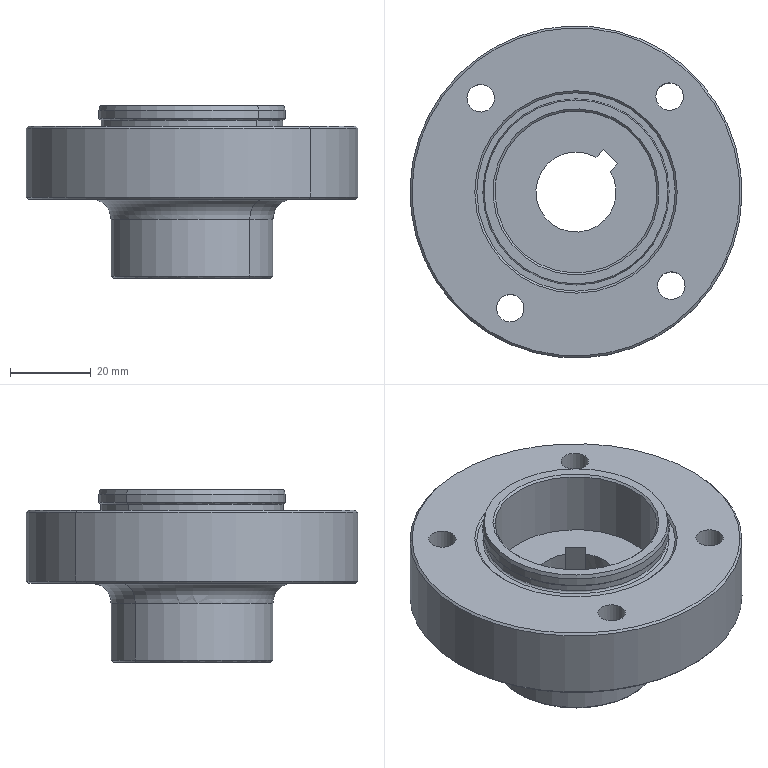Part | SolidWorks | features BaseBody 1 | 1 solid | 48 faces | box 82 x 82 x 42.5 mm | volume 94229 mm3 | cylinder 18 | cone 17 | plane 9 | torus 4 | commonest cylinder face diameters 6.8 x8 40 x4 45 x2 46 x2 82 x2
STEP:
#1=CARTESIAN_POINT('',(-51.524,-43.165,125.25));
#2=VERTEX_POINT('',#1);
#3=CARTESIAN_POINT('',(-37.402,-57.043,125.25));
#4=VERTEX_POINT('',#3);
#5=CARTESIAN_POINT('',(-44.463,-50.104,125.25));
#6=DIRECTION('',(0.,0.,1.));
#7=DIRECTION('',(0.7133,-0.7009,0.));
#8=AXIS2_PLACEMENT_3D('',#5,#6,#7);
#9=CIRCLE('',#8,9.9);
#10=EDGE_CURVE('',#2,#4,#9,.T.);
#11=ORIENTED_EDGE('',*,*,#10,.T.);
#12=CARTESIAN_POINT('',(-35.547,-58.865,99.25));
#13=VERTEX_POINT('',#12);
#14=CARTESIAN_POINT('',(-37.402,-57.043,125.25));
#15=DIRECTION('',(0.07097,-0.06974,-0.995));
#16=VECTOR('',#15,1000.);
#17=LINE('',#14,#16);
#18=EDGE_CURVE('',#4,#13,#17,.T.);
#19=ORIENTED_EDGE('',*,*,#18,.T.);
#20=CARTESIAN_POINT('',(-53.379,-41.342,99.25));
#21=VERTEX_POINT('',#20);
#22=CARTESIAN_POINT('',(-44.463,-50.104,99.25));
#23=DIRECTION('',(0.,0.,1.));
#24=DIRECTION('',(0.7133,-0.7009,0.));
#25=AXIS2_PLACEMENT_3D('',#22,#23,#24);
#26=CIRCLE('',#25,12.5);
#27=EDGE_CURVE('',#21,#13,#26,.T.);
#28=ORIENTED_EDGE('',*,*,#27,.F.);
#29=CARTESIAN_POINT('',(-51.524,-43.165,125.25));
#30=DIRECTION('',(-0.07097,0.06974,-0.995));
#31=VECTOR('',#30,1000.);
#32=LINE('',#29,#31);
#33=EDGE_CURVE('',#2,#21,#32,.T.);
#34=ORIENTED_EDGE('',*,*,#33,.F.);
#35=EDGE_LOOP('',(#11,#19,#28,#34));
#36=FACE_OUTER_BOUND('',#35,.T.);
#37=CARTESIAN_POINT('',(-44.463,-50.104,125.25));
#38=DIRECTION('',(0.,0.,-1.));
#39=DIRECTION('',(-0.7133,0.7009,0.));
#40=AXIS2_PLACEMENT_3D('',#37,#38,#39);
#41=CONICAL_SURFACE('',#40,9.9,0.09967);
#42=ADVANCED_FACE('',(#36),#41,.F.);
#43=CARTESIAN_POINT('',(-39.532,-41.519,125.25));
#44=VERTEX_POINT('',#43);
#45=CARTESIAN_POINT('',(-44.463,-50.104,125.25));
#46=DIRECTION('',(0.,0.,1.));
#47=DIRECTION('',(0.7133,-0.7009,0.));
#48=AXIS2_PLACEMENT_3D('',#45,#46,#47);
#49=CIRCLE('',#48,9.9);
#50=EDGE_CURVE('',#44,#2,#49,.T.);
#51=ORIENTED_EDGE('',*,*,#50,.T.);
#52=ORIENTED_EDGE('',*,*,#33,.T.);
#53=CARTESIAN_POINT('',(-37.662,-39.616,99.25));
#54=VERTEX_POINT('',#53);
#55=CARTESIAN_POINT('',(-44.463,-50.104,99.25));
#56=DIRECTION('',(0.,0.,1.));
#57=DIRECTION('',(0.7133,-0.7009,0.));
#58=AXIS2_PLACEMENT_3D('',#55,#56,#57);
#59=CIRCLE('',#58,12.5);
#60=EDGE_CURVE('',#54,#21,#59,.T.);
#61=ORIENTED_EDGE('',*,*,#60,.F.);
#62=CARTESIAN_POINT('',(-37.662,-39.616,99.25));
#63=CARTESIAN_POINT('',(-38.282,-40.247,107.917));
#64=CARTESIAN_POINT('',(-38.904,-40.88,116.584));
#65=CARTESIAN_POINT('',(-39.532,-41.519,125.25));
#66=B_SPLINE_CURVE_WITH_KNOTS('',3,(#62,#63,#64,#65),.UNSPECIFIED.,.F.,.F.,(4,4),(0.,0.02614),.UNSPECIFIED.);
#67=EDGE_CURVE('',#54,#44,#66,.T.);
#68=ORIENTED_EDGE('',*,*,#67,.T.);
#69=EDGE_LOOP('',(#51,#52,#61,#68));
#70=FACE_OUTER_BOUND('',#69,.T.);
#71=CARTESIAN_POINT('',(-44.463,-50.104,125.25));
#72=DIRECTION('',(0.,0.,-1.));
#73=DIRECTION('',(-0.7133,0.7009,0.));
#74=AXIS2_PLACEMENT_3D('',#71,#72,#73);
#75=CONICAL_SURFACE('',#74,9.9,0.09967);
#76=ADVANCED_FACE('',(#70),#75,.F.);
#77=CARTESIAN_POINT('',(-58.728,-36.086,125.25));
#78=VERTEX_POINT('',#77);
#79=CARTESIAN_POINT('',(-30.198,-64.122,125.25));
#80=VERTEX_POINT('',#79);
#81=CARTESIAN_POINT('',(-44.463,-50.104,125.25));
#82=DIRECTION('',(0.,0.,1.));
#83=DIRECTION('',(0.7133,-0.7009,0.));
#84=AXIS2_PLACEMENT_3D('',#81,#82,#83);
#85=CIRCLE('',#84,20.);
#86=EDGE_CURVE('',#78,#80,#85,.T.);
#87=ORIENTED_EDGE('',*,*,#86,.F.);
#88=CARTESIAN_POINT('',(-58.728,-36.086,141.25));
#89=VERTEX_POINT('',#88);
#90=CARTESIAN_POINT('',(-58.728,-36.086,146.313));
#91=DIRECTION('',(0.,0.,1.));
#92=VECTOR('',#91,1000.);
#93=LINE('',#90,#92);
#94=EDGE_CURVE('',#78,#89,#93,.T.);
#95=ORIENTED_EDGE('',*,*,#94,.T.);
#96=CARTESIAN_POINT('',(-30.198,-64.122,141.25));
#97=VERTEX_POINT('',#96);
#98=CARTESIAN_POINT('',(-44.463,-50.104,141.25));
#99=DIRECTION('',(0.,0.,1.));
#100=DIRECTION('',(0.7133,-0.7009,0.));
#101=AXIS2_PLACEMENT_3D('',#98,#99,#100);
#102=CIRCLE('',#101,20.);
#103=EDGE_CURVE('',#89,#97,#102,.T.);
#104=ORIENTED_EDGE('',*,*,#103,.T.);
#105=CARTESIAN_POINT('',(-30.198,-64.122,146.313));
#106=DIRECTION('',(0.,0.,1.));
#107=VECTOR('',#106,1000.);
#108=LINE('',#105,#107);
#109=EDGE_CURVE('',#80,#97,#108,.T.);
#110=ORIENTED_EDGE('',*,*,#109,.F.);
#111=EDGE_LOOP('',(#87,#95,#104,#110));
#112=FACE_OUTER_BOUND('',#111,.T.);
#113=CARTESIAN_POINT('',(-44.463,-50.104,146.313));
#114=DIRECTION('',(0.,0.,1.));
#115=DIRECTION('',(0.7133,-0.7009,0.));
#116=AXIS2_PLACEMENT_3D('',#113,#114,#115);
#117=CYLINDRICAL_SURFACE('',#116,20.);
#118=ADVANCED_FACE('',(#112),#117,.F.);
#119=ORIENTED_EDGE('',*,*,#103,.F.);
#120=CARTESIAN_POINT('',(-59.085,-35.735,141.75));
#121=VERTEX_POINT('',#120);
#122=CARTESIAN_POINT('',(-59.085,-35.735,141.75));
#123=DIRECTION('',(-0.5043,0.4956,0.7071));
#124=VECTOR('',#123,1000.);
#125=LINE('',#122,#124);
#126=EDGE_CURVE('',#89,#121,#125,.T.);
#127=ORIENTED_EDGE('',*,*,#126,.T.);
#128=CARTESIAN_POINT('',(-29.841,-64.472,141.75));
#129=VERTEX_POINT('',#128);
#130=CARTESIAN_POINT('',(-44.463,-50.104,141.75));
#131=DIRECTION('',(0.,0.,1.));
#132=DIRECTION('',(0.7133,-0.7009,0.));
#133=AXIS2_PLACEMENT_3D('',#130,#131,#132);
#134=CIRCLE('',#133,20.5);
#135=EDGE_CURVE('',#121,#129,#134,.T.);
#136=ORIENTED_EDGE('',*,*,#135,.T.);
#137=CARTESIAN_POINT('',(-29.841,-64.472,141.75));
#138=DIRECTION('',(0.5043,-0.4956,0.7071));
#139=VECTOR('',#138,1000.);
#140=LINE('',#137,#139);
#141=EDGE_CURVE('',#97,#129,#140,.T.);
#142=ORIENTED_EDGE('',*,*,#141,.F.);
#143=EDGE_LOOP('',(#119,#127,#136,#142));
#144=FACE_OUTER_BOUND('',#143,.T.);
#145=CARTESIAN_POINT('',(-44.463,-50.104,141.75));
#146=DIRECTION('',(0.,0.,1.));
#147=DIRECTION('',(0.7133,-0.7009,0.));
#148=AXIS2_PLACEMENT_3D('',#145,#146,#147);
#149=CONICAL_SURFACE('',#148,20.5,0.7854);
#150=ADVANCED_FACE('',(#144),#149,.F.);
#151=CARTESIAN_POINT('',(-28.058,-66.225,138.75));
#152=VERTEX_POINT('',#151);
#153=CARTESIAN_POINT('',(-60.868,-33.983,138.75));
#154=VERTEX_POINT('',#153);
#155=CARTESIAN_POINT('',(-44.463,-50.104,138.75));
#156=DIRECTION('',(0.,0.,1.));
#157=DIRECTION('',(0.7133,-0.7009,0.));
#158=AXIS2_PLACEMENT_3D('',#155,#156,#157);
#159=CIRCLE('',#158,23.);
#160=EDGE_CURVE('',#152,#154,#159,.T.);
#161=ORIENTED_EDGE('',*,*,#160,.T.);
#162=CARTESIAN_POINT('',(-60.868,-33.983,140.75));
#163=VERTEX_POINT('',#162);
#164=CARTESIAN_POINT('',(-60.868,-33.983,146.313));
#165=DIRECTION('',(0.,0.,1.));
#166=VECTOR('',#165,1000.);
#167=LINE('',#164,#166);
#168=EDGE_CURVE('',#154,#163,#167,.T.);
#169=ORIENTED_EDGE('',*,*,#168,.T.);
#170=CARTESIAN_POINT('',(-28.058,-66.225,140.75));
#171=VERTEX_POINT('',#170);
#172=CARTESIAN_POINT('',(-44.463,-50.104,140.75));
#173=DIRECTION('',(0.,0.,-1.));
#174=DIRECTION('',(-0.7133,0.7009,0.));
#175=AXIS2_PLACEMENT_3D('',#172,#173,#174);
#176=CIRCLE('',#175,23.);
#177=EDGE_CURVE('',#163,#171,#176,.T.);
#178=ORIENTED_EDGE('',*,*,#177,.T.);
#179=CARTESIAN_POINT('',(-28.058,-66.225,146.313));
#180=DIRECTION('',(0.,0.,1.));
#181=VECTOR('',#180,1000.);
#182=LINE('',#179,#181);
#183=EDGE_CURVE('',#152,#171,#182,.T.);
#184=ORIENTED_EDGE('',*,*,#183,.F.);
#185=EDGE_LOOP('',(#161,#169,#178,#184));
#186=FACE_OUTER_BOUND('',#185,.T.);
#187=CARTESIAN_POINT('',(-44.463,-50.104,146.313));
#188=DIRECTION('',(0.,0.,1.));
#189=DIRECTION('',(0.7133,-0.7009,0.));
#190=AXIS2_PLACEMENT_3D('',#187,#188,#189);
#191=CYLINDRICAL_SURFACE('',#190,23.);
#192=ADVANCED_FACE('',(#186),#191,.T.);
#193=CARTESIAN_POINT('',(-28.415,-65.874,138.25));
#194=VERTEX_POINT('',#193);
#195=CARTESIAN_POINT('',(-60.511,-34.333,138.25));
#196=VERTEX_POINT('',#195);
#197=CARTESIAN_POINT('',(-44.463,-50.104,138.25));
#198=DIRECTION('',(0.,0.,1.));
#199=DIRECTION('',(0.7133,-0.7009,0.));
#200=AXIS2_PLACEMENT_3D('',#197,#198,#199);
#201=CIRCLE('',#200,22.5);
#202=EDGE_CURVE('',#194,#196,#201,.T.);
#203=ORIENTED_EDGE('',*,*,#202,.T.);
#204=CARTESIAN_POINT('',(-60.511,-34.333,138.25));
#205=DIRECTION('',(-0.5043,0.4956,0.7071));
#206=VECTOR('',#205,1000.);
#207=LINE('',#204,#206);
#208=EDGE_CURVE('',#196,#154,#207,.T.);
#209=ORIENTED_EDGE('',*,*,#208,.T.);
#210=ORIENTED_EDGE('',*,*,#160,.F.);
#211=CARTESIAN_POINT('',(-28.415,-65.874,138.25));
#212=DIRECTION('',(0.5043,-0.4956,0.7071));
#213=VECTOR('',#212,1000.);
#214=LINE('',#211,#213);
#215=EDGE_CURVE('',#194,#152,#214,.T.);
#216=ORIENTED_EDGE('',*,*,#215,.F.);
#217=EDGE_LOOP('',(#203,#209,#210,#216));
#218=FACE_OUTER_BOUND('',#217,.T.);
#219=CARTESIAN_POINT('',(-44.463,-50.104,138.25));
#220=DIRECTION('',(0.,0.,1.));
#221=DIRECTION('',(0.7133,-0.7009,0.));
#222=AXIS2_PLACEMENT_3D('',#219,#220,#221);
#223=CONICAL_SURFACE('',#222,22.5,0.7854);
#224=ADVANCED_FACE('',(#218),#223,.T.);
#225=CARTESIAN_POINT('',(-28.415,-65.874,136.75));
#226=VERTEX_POINT('',#225);
#227=CARTESIAN_POINT('',(-60.511,-34.333,136.75));
#228=VERTEX_POINT('',#227);
#229=CARTESIAN_POINT('',(-44.463,-50.104,136.75));
#230=DIRECTION('',(0.,0.,1.));
#231=DIRECTION('',(-0.7133,0.7009,0.));
#232=AXIS2_PLACEMENT_3D('',#229,#230,#231);
#233=CIRCLE('',#232,22.5);
#234=EDGE_CURVE('',#226,#228,#233,.T.);
#235=ORIENTED_EDGE('',*,*,#234,.T.);
#236=CARTESIAN_POINT('',(-60.511,-34.333,146.313));
#237=DIRECTION('',(0.,0.,1.));
#238=VECTOR('',#237,1000.);
#239=LINE('',#236,#238);
#240=EDGE_CURVE('',#228,#196,#239,.T.);
#241=ORIENTED_EDGE('',*,*,#240,.T.);
#242=ORIENTED_EDGE('',*,*,#202,.F.);
#243=CARTESIAN_POINT('',(-28.415,-65.874,146.313));
#244=DIRECTION('',(0.,0.,1.));
#245=VECTOR('',#244,1000.);
#246=LINE('',#243,#245);
#247=EDGE_CURVE('',#226,#194,#246,.T.);
#248=ORIENTED_EDGE('',*,*,#247,.F.);
#249=EDGE_LOOP('',(#235,#241,#242,#248));
#250=FACE_OUTER_BOUND('',#249,.T.);
#251=CARTESIAN_POINT('',(-44.463,-50.104,146.313));
#252=DIRECTION('',(0.,0.,1.));
#253=DIRECTION('',(0.7133,-0.7009,0.));
#254=AXIS2_PLACEMENT_3D('',#251,#252,#253);
#255=CYLINDRICAL_SURFACE('',#254,22.5);
#256=ADVANCED_FACE('',(#250),#255,.T.);
#257=CARTESIAN_POINT('',(-61.938,-32.932,136.25));
#258=VERTEX_POINT('',#257);
#259=CARTESIAN_POINT('',(-26.988,-67.276,136.25));
#260=VERTEX_POINT('',#259);
#261=CARTESIAN_POINT('',(-44.463,-50.104,136.25));
#262=DIRECTION('',(0.,0.,1.));
#263=DIRECTION('',(0.7133,-0.7009,0.));
#264=AXIS2_PLACEMENT_3D('',#261,#262,#263);
#265=CIRCLE('',#264,24.5);
#266=EDGE_CURVE('',#258,#260,#265,.T.);
#267=ORIENTED_EDGE('',*,*,#266,.F.);
#268=CARTESIAN_POINT('',(-62.294,-32.581,136.75));
#269=VERTEX_POINT('',#268);
#270=CARTESIAN_POINT('',(-62.294,-32.581,136.75));
#271=DIRECTION('',(-0.5043,0.4956,0.7071));
#272=VECTOR('',#271,1000.);
#273=LINE('',#270,#272);
#274=EDGE_CURVE('',#258,#269,#273,.T.);
#275=ORIENTED_EDGE('',*,*,#274,.T.);
#276=CARTESIAN_POINT('',(-26.632,-67.627,136.75));
#277=VERTEX_POINT('',#276);
#278=CARTESIAN_POINT('',(-44.463,-50.104,136.75));
#279=DIRECTION('',(0.,0.,1.));
#280=DIRECTION('',(0.7133,-0.7009,0.));
#281=AXIS2_PLACEMENT_3D('',#278,#279,#280);
#282=CIRCLE('',#281,25.);
#283=EDGE_CURVE('',#269,#277,#282,.T.);
#284=ORIENTED_EDGE('',*,*,#283,.T.);
#285=CARTESIAN_POINT('',(-26.632,-67.627,136.75));
#286=DIRECTION('',(0.5043,-0.4956,0.7071));
#287=VECTOR('',#286,1000.);
#288=LINE('',#285,#287);
#289=EDGE_CURVE('',#260,#277,#288,.T.);
#290=ORIENTED_EDGE('',*,*,#289,.F.);
#291=EDGE_LOOP('',(#267,#275,#284,#290));
#292=FACE_OUTER_BOUND('',#291,.T.);
#293=CARTESIAN_POINT('',(-44.463,-50.104,136.75));
#294=DIRECTION('',(0.,0.,1.));
#295=DIRECTION('',(0.7133,-0.7009,0.));
#296=AXIS2_PLACEMENT_3D('',#293,#294,#295);
#297=CONICAL_SURFACE('',#296,25.,0.7854);
#298=ADVANCED_FACE('',(#292),#297,.F.);
#299=CARTESIAN_POINT('',(-15.22,-78.841,119.25));
#300=VERTEX_POINT('',#299);
#301=CARTESIAN_POINT('',(-73.706,-21.366,119.25));
#302=VERTEX_POINT('',#301);
#303=CARTESIAN_POINT('',(-44.463,-50.104,119.25));
#304=DIRECTION('',(0.,0.,1.));
#305=DIRECTION('',(0.7133,-0.7009,0.));
#306=AXIS2_PLACEMENT_3D('',#303,#304,#305);
#307=CIRCLE('',#306,41.);
#308=EDGE_CURVE('',#300,#302,#307,.T.);
#309=ORIENTED_EDGE('',*,*,#308,.T.);
#310=CARTESIAN_POINT('',(-73.706,-21.366,136.25));
#311=VERTEX_POINT('',#310);
#312=CARTESIAN_POINT('',(-73.706,-21.366,146.313));
#313=DIRECTION('',(0.,0.,1.));
#314=VECTOR('',#313,1000.);
#315=LINE('',#312,#314);
#316=EDGE_CURVE('',#302,#311,#315,.T.);
#317=ORIENTED_EDGE('',*,*,#316,.T.);
#318=CARTESIAN_POINT('',(-15.22,-78.841,136.25));
#319=VERTEX_POINT('',#318);
#320=CARTESIAN_POINT('',(-44.463,-50.104,136.25));
#321=DIRECTION('',(0.,0.,-1.));
#322=DIRECTION('',(-0.7133,0.7009,0.));
#323=AXIS2_PLACEMENT_3D('',#320,#321,#322);
#324=CIRCLE('',#323,41.);
#325=EDGE_CURVE('',#311,#319,#324,.T.);
#326=ORIENTED_EDGE('',*,*,#325,.T.);
#327=CARTESIAN_POINT('',(-15.22,-78.841,146.313));
#328=DIRECTION('',(0.,0.,1.));
#329=VECTOR('',#328,1000.);
#330=LINE('',#327,#329);
#331=EDGE_CURVE('',#300,#319,#330,.T.);
#332=ORIENTED_EDGE('',*,*,#331,.F.);
#333=EDGE_LOOP('',(#309,#317,#326,#332));
#334=FACE_OUTER_BOUND('',#333,.T.);
#335=CARTESIAN_POINT('',(-44.463,-50.104,146.313));
#336=DIRECTION('',(0.,0.,1.));
#337=DIRECTION('',(0.7133,-0.7009,0.));
#338=AXIS2_PLACEMENT_3D('',#335,#336,#337);
#339=CYLINDRICAL_SURFACE('',#338,41.);
#340=ADVANCED_FACE('',(#334),#339,.T.);
#341=CARTESIAN_POINT('',(-62.294,-32.581,118.75));
#342=VERTEX_POINT('',#341);
#343=CARTESIAN_POINT('',(-26.632,-67.627,118.75));
#344=VERTEX_POINT('',#343);
#345=CARTESIAN_POINT('',(-44.463,-50.104,118.75));
#346=DIRECTION('',(0.,0.,1.));
#347=DIRECTION('',(0.7133,-0.7009,0.));
#348=AXIS2_PLACEMENT_3D('',#345,#346,#347);
#349=CIRCLE('',#348,25.);
#350=EDGE_CURVE('',#342,#344,#349,.T.);
#351=ORIENTED_EDGE('',*,*,#350,.F.);
#352=CARTESIAN_POINT('',(-58.728,-36.086,113.75));
#353=VERTEX_POINT('',#352);
#354=CARTESIAN_POINT('',(-62.294,-32.581,113.75));
#355=DIRECTION('',(0.7009,0.7133,0.));
#356=DIRECTION('',(-0.7133,0.7009,0.));
#357=AXIS2_PLACEMENT_3D('',#354,#355,#356);
#358=CIRCLE('',#357,5.);
#359=EDGE_CURVE('',#342,#353,#358,.T.);
#360=ORIENTED_EDGE('',*,*,#359,.T.);
#361=CARTESIAN_POINT('',(-30.198,-64.122,113.75));
#362=VERTEX_POINT('',#361);
#363=CARTESIAN_POINT('',(-44.463,-50.104,113.75));
#364=DIRECTION('',(0.,0.,1.));
#365=DIRECTION('',(0.7133,-0.7009,0.));
#366=AXIS2_PLACEMENT_3D('',#363,#364,#365);
#367=CIRCLE('',#366,20.);
#368=EDGE_CURVE('',#353,#362,#367,.T.);
#369=ORIENTED_EDGE('',*,*,#368,.T.);
#370=CARTESIAN_POINT('',(-26.632,-67.627,113.75));
#371=DIRECTION('',(-0.7009,-0.7133,0.));
#372=DIRECTION('',(0.7133,-0.7009,0.));
#373=AXIS2_PLACEMENT_3D('',#370,#371,#372);
#374=CIRCLE('',#373,5.);
#375=EDGE_CURVE('',#344,#362,#374,.T.);
#376=ORIENTED_EDGE('',*,*,#375,.F.);
#377=EDGE_LOOP('',(#351,#360,#369,#376));
#378=FACE_OUTER_BOUND('',#377,.T.);
#379=CARTESIAN_POINT('',(-44.463,-50.104,113.75));
#380=DIRECTION('',(0.,0.,1.));
#381=DIRECTION('',(0.7133,-0.7009,0.));
#382=AXIS2_PLACEMENT_3D('',#379,#380,#381);
#383=TOROIDAL_SURFACE('',#382,25.,5.);
#384=ADVANCED_FACE('',(#378),#383,.F.);
#385=CARTESIAN_POINT('',(-30.198,-64.122,99.75));
#386=VERTEX_POINT('',#385);
#387=CARTESIAN_POINT('',(-58.728,-36.086,99.75));
#388=VERTEX_POINT('',#387);
#389=CARTESIAN_POINT('',(-44.463,-50.104,99.75));
#390=DIRECTION('',(0.,0.,1.));
#391=DIRECTION('',(0.7133,-0.7009,0.));
#392=AXIS2_PLACEMENT_3D('',#389,#390,#391);
#393=CIRCLE('',#392,20.);
#394=EDGE_CURVE('',#386,#388,#393,.T.);
#395=ORIENTED_EDGE('',*,*,#394,.T.);
#396=CARTESIAN_POINT('',(-58.728,-36.086,146.313));
#397=DIRECTION('',(0.,0.,1.));
#398=VECTOR('',#397,1000.);
#399=LINE('',#396,#398);
#400=EDGE_CURVE('',#388,#353,#399,.T.);
#401=ORIENTED_EDGE('',*,*,#400,.T.);
#402=CARTESIAN_POINT('',(-44.463,-50.104,113.75));
#403=DIRECTION('',(0.,0.,1.));
#404=DIRECTION('',(0.7133,-0.7009,0.));
#405=AXIS2_PLACEMENT_3D('',#402,#403,#404);
#406=CIRCLE('',#405,20.);
#407=EDGE_CURVE('',#362,#353,#406,.T.);
#408=ORIENTED_EDGE('',*,*,#407,.F.);
#409=CARTESIAN_POINT('',(-30.198,-64.122,146.313));
#410=DIRECTION('',(0.,0.,1.));
#411=VECTOR('',#410,1000.);
#412=LINE('',#409,#411);
#413=EDGE_CURVE('',#386,#362,#412,.T.);
#414=ORIENTED_EDGE('',*,*,#413,.F.);
#415=EDGE_LOOP('',(#395,#401,#408,#414));
#416=FACE_OUTER_BOUND('',#415,.T.);
#417=CARTESIAN_POINT('',(-44.463,-50.104,146.313));
#418=DIRECTION('',(0.,0.,1.));
#419=DIRECTION('',(0.7133,-0.7009,0.));
#420=AXIS2_PLACEMENT_3D('',#417,#418,#419);
#421=CYLINDRICAL_SURFACE('',#420,20.);
#422=ADVANCED_FACE('',(#416),#421,.T.);
#423=CARTESIAN_POINT('',(-58.371,-36.436,99.25));
#424=VERTEX_POINT('',#423);
#425=CARTESIAN_POINT('',(-30.554,-63.772,99.25));
#426=VERTEX_POINT('',#425);
#427=CARTESIAN_POINT('',(-44.463,-50.104,99.25));
#428=DIRECTION('',(0.,0.,-1.));
#429=DIRECTION('',(0.7133,-0.7009,0.));
#430=AXIS2_PLACEMENT_3D('',#427,#428,#429);
#431=CIRCLE('',#430,19.5);
#432=EDGE_CURVE('',#424,#426,#431,.T.);
#433=ORIENTED_EDGE('',*,*,#432,.F.);
#434=CARTESIAN_POINT('',(-58.728,-36.086,99.75));
#435=DIRECTION('',(-0.5043,0.4956,0.7071));
#436=VECTOR('',#435,1000.);
#437=LINE('',#434,#436);
#438=EDGE_CURVE('',#424,#388,#437,.T.);
#439=ORIENTED_EDGE('',*,*,#438,.T.);
#440=ORIENTED_EDGE('',*,*,#394,.F.);
#441=CARTESIAN_POINT('',(-30.198,-64.122,99.75));
#442=DIRECTION('',(0.5043,-0.4956,0.7071));
#443=VECTOR('',#442,1000.);
#444=LINE('',#441,#443);
#445=EDGE_CURVE('',#426,#386,#444,.T.);
#446=ORIENTED_EDGE('',*,*,#445,.F.);
#447=EDGE_LOOP('',(#433,#439,#440,#446));
#448=FACE_OUTER_BOUND('',#447,.T.);
#449=CARTESIAN_POINT('',(-44.463,-50.104,99.75));
#450=DIRECTION('',(0.,0.,1.));
#451=DIRECTION('',(0.7133,-0.7009,0.));
#452=AXIS2_PLACEMENT_3D('',#449,#450,#451);
#453=CONICAL_SURFACE('',#452,20.,0.7854);
#454=ADVANCED_FACE('',(#448),#453,.T.);
#455=CARTESIAN_POINT('',(-73.35,-21.717,118.75));
#456=VERTEX_POINT('',#455);
#457=CARTESIAN_POINT('',(-15.576,-78.491,118.75));
#458=VERTEX_POINT('',#457);
#459=CARTESIAN_POINT('',(-44.463,-50.104,118.75));
#460=DIRECTION('',(0.,0.,-1.));
#461=DIRECTION('',(0.7133,-0.7009,0.));
#462=AXIS2_PLACEMENT_3D('',#459,#460,#461);
#463=CIRCLE('',#462,40.5);
#464=EDGE_CURVE('',#456,#458,#463,.T.);
#465=ORIENTED_EDGE('',*,*,#464,.F.);
#466=CARTESIAN_POINT('',(-73.706,-21.366,119.25));
#467=DIRECTION('',(-0.5043,0.4956,0.7071));
#468=VECTOR('',#467,1000.);
#469=LINE('',#466,#468);
#470=EDGE_CURVE('',#456,#302,#469,.T.);
#471=ORIENTED_EDGE('',*,*,#470,.T.);
#472=ORIENTED_EDGE('',*,*,#308,.F.);
#473=CARTESIAN_POINT('',(-15.22,-78.841,119.25));
#474=DIRECTION('',(0.5043,-0.4956,0.7071));
#475=VECTOR('',#474,1000.);
#476=LINE('',#473,#475);
#477=EDGE_CURVE('',#458,#300,#476,.T.);
#478=ORIENTED_EDGE('',*,*,#477,.F.);
#479=EDGE_LOOP('',(#465,#471,#472,#478));
#480=FACE_OUTER_BOUND('',#479,.T.);
#481=CARTESIAN_POINT('',(-44.463,-50.104,119.25));
#482=DIRECTION('',(0.,0.,1.));
#483=DIRECTION('',(0.7133,-0.7009,0.));
#484=AXIS2_PLACEMENT_3D('',#481,#482,#483);
#485=CONICAL_SURFACE('',#484,41.,0.7854);
#486=ADVANCED_FACE('',(#480),#485,.T.);
#487=CARTESIAN_POINT('',(-15.576,-78.491,136.75));
#488=VERTEX_POINT('',#487);
#489=CARTESIAN_POINT('',(-73.35,-21.717,136.75));
#490=VERTEX_POINT('',#489);
#491=CARTESIAN_POINT('',(-44.463,-50.104,136.75));
#492=DIRECTION('',(0.,0.,1.));
#493=DIRECTION('',(-0.7133,0.7009,0.));
#494=AXIS2_PLACEMENT_3D('',#491,#492,#493);
#495=CIRCLE('',#494,40.5);
#496=EDGE_CURVE('',#488,#490,#495,.T.);
#497=ORIENTED_EDGE('',*,*,#496,.F.);
#498=CARTESIAN_POINT('',(-15.576,-78.491,136.75));
#499=DIRECTION('',(0.5043,-0.4956,-0.7071));
#500=VECTOR('',#499,1000.);
#501=LINE('',#498,#500);
#502=EDGE_CURVE('',#488,#319,#501,.T.);
#503=ORIENTED_EDGE('',*,*,#502,.T.);
#504=ORIENTED_EDGE('',*,*,#325,.F.);
#505=CARTESIAN_POINT('',(-73.35,-21.717,136.75));
#506=DIRECTION('',(-0.5043,0.4956,-0.7071));
#507=VECTOR('',#506,1000.);
#508=LINE('',#505,#507);
#509=EDGE_CURVE('',#490,#311,#508,.T.);
#510=ORIENTED_EDGE('',*,*,#509,.F.);
#511=EDGE_LOOP('',(#497,#503,#504,#510));
#512=FACE_OUTER_BOUND('',#511,.T.);
#513=CARTESIAN_POINT('',(-44.463,-50.104,136.75));
#514=DIRECTION('',(0.,0.,-1.));
#515=DIRECTION('',(-0.7133,0.7009,0.));
#516=AXIS2_PLACEMENT_3D('',#513,#514,#515);
#517=CONICAL_SURFACE('',#516,40.5,0.7854);
#518=ADVANCED_FACE('',(#512),#517,.T.);
#519=CARTESIAN_POINT('',(-28.058,-66.225,136.25));
#520=VERTEX_POINT('',#519);
#521=CARTESIAN_POINT('',(-60.868,-33.983,136.25));
#522=VERTEX_POINT('',#521);
#523=CARTESIAN_POINT('',(-44.463,-50.104,136.25));
#524=DIRECTION('',(0.,0.,-1.));
#525=DIRECTION('',(-0.7133,0.7009,0.));
#526=AXIS2_PLACEMENT_3D('',#523,#524,#525);
#527=CIRCLE('',#526,23.);
#528=EDGE_CURVE('',#520,#522,#527,.T.);
#529=ORIENTED_EDGE('',*,*,#528,.F.);
#530=CARTESIAN_POINT('',(-28.058,-66.225,136.75));
#531=DIRECTION('',(0.7009,0.7133,0.));
#532=DIRECTION('',(-0.7133,0.7009,0.));
#533=AXIS2_PLACEMENT_3D('',#530,#531,#532);
#534=CIRCLE('',#533,0.5);
#535=EDGE_CURVE('',#520,#226,#534,.T.);
#536=ORIENTED_EDGE('',*,*,#535,.T.);
#537=CARTESIAN_POINT('',(-44.463,-50.104,136.75));
#538=DIRECTION('',(0.,0.,1.));
#539=DIRECTION('',(-0.7133,0.7009,0.));
#540=AXIS2_PLACEMENT_3D('',#537,#538,#539);
#541=CIRCLE('',#540,22.5);
#542=EDGE_CURVE('',#228,#226,#541,.T.);
#543=ORIENTED_EDGE('',*,*,#542,.F.);
#544=CARTESIAN_POINT('',(-60.868,-33.983,136.75));
#545=DIRECTION('',(-0.7009,-0.7133,0.));
#546=DIRECTION('',(0.7133,-0.7009,0.));
#547=AXIS2_PLACEMENT_3D('',#544,#545,#546);
#548=CIRCLE('',#547,0.5);
#549=EDGE_CURVE('',#522,#228,#548,.T.);
#550=ORIENTED_EDGE('',*,*,#549,.F.);
#551=EDGE_LOOP('',(#529,#536,#543,#550));
#552=FACE_OUTER_BOUND('',#551,.T.);
#553=CARTESIAN_POINT('',(-44.463,-50.104,136.75));
#554=DIRECTION('',(0.,0.,-1.));
#555=DIRECTION('',(-0.7133,0.7009,0.));
#556=AXIS2_PLACEMENT_3D('',#553,#554,#555);
#557=TOROIDAL_SURFACE('',#556,23.,0.5);
#558=ADVANCED_FACE('',(#552),#557,.F.);
#559=CARTESIAN_POINT('',(-18.501,-75.617,136.75));
#560=VERTEX_POINT('',#559);
#561=CARTESIAN_POINT('',(-23.351,-70.851,136.75));
#562=VERTEX_POINT('',#561);
#563=CARTESIAN_POINT('',(-20.926,-73.234,136.75));
#564=DIRECTION('',(0.,0.,-1.));
#565=DIRECTION('',(-0.7133,0.7009,0.));
#566=AXIS2_PLACEMENT_3D('',#563,#564,#565);
#567=CIRCLE('',#566,3.4);
#568=EDGE_CURVE('',#560,#562,#567,.T.);
#569=ORIENTED_EDGE('',*,*,#568,.F.);
#570=CARTESIAN_POINT('',(-18.501,-75.617,118.75));
#571=VERTEX_POINT('',#570);
#572=CARTESIAN_POINT('',(-18.501,-75.617,118.75));
#573=DIRECTION('',(0.,0.,-1.));
#574=VECTOR('',#573,1000.);
#575=LINE('',#572,#574);
#576=EDGE_CURVE('',#560,#571,#575,.T.);
#577=ORIENTED_EDGE('',*,*,#576,.T.);
#578=CARTESIAN_POINT('',(-23.351,-70.851,118.75));
#579=VERTEX_POINT('',#578);
#580=CARTESIAN_POINT('',(-20.926,-73.234,118.75));
#581=DIRECTION('',(0.,0.,-1.));
#582=DIRECTION('',(-0.7133,0.7009,0.));
#583=AXIS2_PLACEMENT_3D('',#580,#581,#582);
#584=CIRCLE('',#583,3.4);
#585=EDGE_CURVE('',#571,#579,#584,.T.);
#586=ORIENTED_EDGE('',*,*,#585,.T.);
#587=CARTESIAN_POINT('',(-23.351,-70.851,118.75));
#588=DIRECTION('',(0.,0.,-1.));
#589=VECTOR('',#588,1000.);
#590=LINE('',#587,#589);
#591=EDGE_CURVE('',#562,#579,#590,.T.);
#592=ORIENTED_EDGE('',*,*,#591,.F.);
#593=EDGE_LOOP('',(#569,#577,#586,#592));
#594=FACE_OUTER_BOUND('',#593,.T.);
#595=CARTESIAN_POINT('',(-20.926,-73.234,118.75));
#596=DIRECTION('',(0.,0.,-1.));
#597=DIRECTION('',(-0.7133,0.7009,0.));
#598=AXIS2_PLACEMENT_3D('',#595,#596,#597);
#599=CYLINDRICAL_SURFACE('',#598,3.4);
#600=ADVANCED_FACE('',(#594),#599,.F.);
#601=CARTESIAN_POINT('',(-18.908,-28.95,136.75));
#602=VERTEX_POINT('',#601);
#603=CARTESIAN_POINT('',(-23.758,-24.183,136.75));
#604=VERTEX_POINT('',#603);
#605=CARTESIAN_POINT('',(-21.333,-26.567,136.75));
#606=DIRECTION('',(0.,0.,-1.));
#607=DIRECTION('',(-0.7133,0.7009,0.));
#608=AXIS2_PLACEMENT_3D('',#605,#606,#607);
#609=CIRCLE('',#608,3.4);
#610=EDGE_CURVE('',#602,#604,#609,.T.);
#611=ORIENTED_EDGE('',*,*,#610,.F.);
#612=CARTESIAN_POINT('',(-18.908,-28.95,118.75));
#613=VERTEX_POINT('',#612);
#614=CARTESIAN_POINT('',(-18.908,-28.95,118.75));
#615=DIRECTION('',(0.,0.,-1.));
#616=VECTOR('',#615,1000.);
#617=LINE('',#614,#616);
#618=EDGE_CURVE('',#602,#613,#617,.T.);
#619=ORIENTED_EDGE('',*,*,#618,.T.);
#620=CARTESIAN_POINT('',(-23.758,-24.183,118.75));
#621=VERTEX_POINT('',#620);
#622=CARTESIAN_POINT('',(-21.333,-26.567,118.75));
#623=DIRECTION('',(0.,0.,-1.));
#624=DIRECTION('',(-0.7133,0.7009,0.));
#625=AXIS2_PLACEMENT_3D('',#622,#623,#624);
#626=CIRCLE('',#625,3.4);
#627=EDGE_CURVE('',#613,#621,#626,.T.);
#628=ORIENTED_EDGE('',*,*,#627,.T.);
#629=CARTESIAN_POINT('',(-23.758,-24.183,118.75));
#630=DIRECTION('',(0.,0.,-1.));
#631=VECTOR('',#630,1000.);
#632=LINE('',#629,#631);
#633=EDGE_CURVE('',#604,#621,#632,.T.);
#634=ORIENTED_EDGE('',*,*,#633,.F.);
#635=EDGE_LOOP('',(#611,#619,#628,#634));
#636=FACE_OUTER_BOUND('',#635,.T.);
#637=CARTESIAN_POINT('',(-21.333,-26.567,118.75));
#638=DIRECTION('',(0.,0.,-1.));
#639=DIRECTION('',(-0.7133,0.7009,0.));
#640=AXIS2_PLACEMENT_3D('',#637,#638,#639);
#641=CYLINDRICAL_SURFACE('',#640,3.4);
#642=ADVANCED_FACE('',(#636),#641,.F.);
#643=CARTESIAN_POINT('',(-65.575,-29.357,136.75));
#644=VERTEX_POINT('',#643);
#645=CARTESIAN_POINT('',(-70.425,-24.591,136.75));
#646=VERTEX_POINT('',#645);
#647=CARTESIAN_POINT('',(-68.,-26.974,136.75));
#648=DIRECTION('',(0.,0.,-1.));
#649=DIRECTION('',(-0.7133,0.7009,0.));
#650=AXIS2_PLACEMENT_3D('',#647,#648,#649);
#651=CIRCLE('',#650,3.4);
#652=EDGE_CURVE('',#644,#646,#651,.T.);
#653=ORIENTED_EDGE('',*,*,#652,.F.);
#654=CARTESIAN_POINT('',(-65.575,-29.357,118.75));
#655=VERTEX_POINT('',#654);
#656=CARTESIAN_POINT('',(-65.575,-29.357,118.75));
#657=DIRECTION('',(0.,0.,-1.));
#658=VECTOR('',#657,1000.);
#659=LINE('',#656,#658);
#660=EDGE_CURVE('',#644,#655,#659,.T.);
#661=ORIENTED_EDGE('',*,*,#660,.T.);
#662=CARTESIAN_POINT('',(-70.425,-24.591,118.75));
#663=VERTEX_POINT('',#662);
#664=CARTESIAN_POINT('',(-68.,-26.974,118.75));
#665=DIRECTION('',(0.,0.,-1.));
#666=DIRECTION('',(-0.7133,0.7009,0.));
#667=AXIS2_PLACEMENT_3D('',#664,#665,#666);
#668=CIRCLE('',#667,3.4);
#669=EDGE_CURVE('',#655,#663,#668,.T.);
#670=ORIENTED_EDGE('',*,*,#669,.T.);
#671=CARTESIAN_POINT('',(-70.425,-24.591,118.75));
#672=DIRECTION('',(0.,0.,-1.));
#673=VECTOR('',#672,1000.);
#674=LINE('',#671,#673);
#675=EDGE_CURVE('',#646,#663,#674,.T.);
#676=ORIENTED_EDGE('',*,*,#675,.F.);
#677=EDGE_LOOP('',(#653,#661,#670,#676));
#678=FACE_OUTER_BOUND('',#677,.T.);
#679=CARTESIAN_POINT('',(-68.,-26.974,118.75));
#680=DIRECTION('',(0.,0.,-1.));
#681=DIRECTION('',(-0.7133,0.7009,0.));
#682=AXIS2_PLACEMENT_3D('',#679,#680,#681);
#683=CYLINDRICAL_SURFACE('',#682,3.4);
#684=ADVANCED_FACE('',(#678),#683,.F.);
#685=CARTESIAN_POINT('',(-58.288,-81.209,136.75));
#686=VERTEX_POINT('',#685);
#687=CARTESIAN_POINT('',(-63.138,-76.442,136.75));
#688=VERTEX_POINT('',#687);
#689=CARTESIAN_POINT('',(-60.713,-78.826,136.75));
#690=DIRECTION('',(0.,0.,-1.));
#691=DIRECTION('',(-0.7133,0.7009,0.));
#692=AXIS2_PLACEMENT_3D('',#689,#690,#691);
#693=CIRCLE('',#692,3.4);
#694=EDGE_CURVE('',#686,#688,#693,.T.);
#695=ORIENTED_EDGE('',*,*,#694,.F.);
#696=CARTESIAN_POINT('',(-58.288,-81.209,118.75));
#697=VERTEX_POINT('',#696);
#698=CARTESIAN_POINT('',(-58.288,-81.209,118.75));
#699=DIRECTION('',(0.,0.,-1.));
#700=VECTOR('',#699,1000.);
#701=LINE('',#698,#700);
#702=EDGE_CURVE('',#686,#697,#701,.T.);
#703=ORIENTED_EDGE('',*,*,#702,.T.);
#704=CARTESIAN_POINT('',(-63.138,-76.442,118.75));
#705=VERTEX_POINT('',#704);
#706=CARTESIAN_POINT('',(-60.713,-78.826,118.75));
#707=DIRECTION('',(0.,0.,-1.));
#708=DIRECTION('',(-0.7133,0.7009,0.));
#709=AXIS2_PLACEMENT_3D('',#706,#707,#708);
#710=CIRCLE('',#709,3.4);
#711=EDGE_CURVE('',#697,#705,#710,.T.);
#712=ORIENTED_EDGE('',*,*,#711,.T.);
#713=CARTESIAN_POINT('',(-63.138,-76.442,118.75));
#714=DIRECTION('',(0.,0.,-1.));
#715=VECTOR('',#714,1000.);
#716=LINE('',#713,#715);
#717=EDGE_CURVE('',#688,#705,#716,.T.);
#718=ORIENTED_EDGE('',*,*,#717,.F.);
#719=EDGE_LOOP('',(#695,#703,#712,#718));
#720=FACE_OUTER_BOUND('',#719,.T.);
#721=CARTESIAN_POINT('',(-60.713,-78.826,118.75));
#722=DIRECTION('',(0.,0.,-1.));
#723=DIRECTION('',(-0.7133,0.7009,0.));
#724=AXIS2_PLACEMENT_3D('',#721,#722,#723);
#725=CYLINDRICAL_SURFACE('',#724,3.4);
#726=ADVANCED_FACE('',(#720),#725,.F.);
#727=CARTESIAN_POINT('',(-28.263,-66.024,141.75));
#728=VERTEX_POINT('',#727);
#729=CARTESIAN_POINT('',(-60.663,-34.184,141.75));
#730=VERTEX_POINT('',#729);
#731=CARTESIAN_POINT('',(-44.463,-50.104,141.75));
#732=DIRECTION('',(0.,0.,1.));
#733=DIRECTION('',(-0.7133,0.7009,0.));
#734=AXIS2_PLACEMENT_3D('',#731,#732,#733);
#735=CIRCLE('',#734,22.713);
#736=EDGE_CURVE('',#728,#730,#735,.T.);
#737=ORIENTED_EDGE('',*,*,#736,.F.);
#738=CARTESIAN_POINT('',(-28.263,-66.024,141.75));
#739=DIRECTION('',(0.1966,-0.1932,-0.9613));
#740=VECTOR('',#739,1000.);
#741=LINE('',#738,#740);
#742=EDGE_CURVE('',#728,#171,#741,.T.);
#743=ORIENTED_EDGE('',*,*,#742,.T.);
#744=ORIENTED_EDGE('',*,*,#177,.F.);
#745=CARTESIAN_POINT('',(-60.663,-34.184,141.75));
#746=DIRECTION('',(-0.1966,0.1932,-0.9613));
#747=VECTOR('',#746,1000.);
#748=LINE('',#745,#747);
#749=EDGE_CURVE('',#730,#163,#748,.T.);
#750=ORIENTED_EDGE('',*,*,#749,.F.);
#751=EDGE_LOOP('',(#737,#743,#744,#750));
#752=FACE_OUTER_BOUND('',#751,.T.);
#753=CARTESIAN_POINT('',(-44.463,-50.104,141.75));
#754=DIRECTION('',(0.,0.,-1.));
#755=DIRECTION('',(-0.7133,0.7009,0.));
#756=AXIS2_PLACEMENT_3D('',#753,#754,#755);
#757=CONICAL_SURFACE('',#756,22.713,0.2793);
#758=ADVANCED_FACE('',(#752),#757,.T.);
#759=ORIENTED_EDGE('',*,*,#742,.F.);
#760=CARTESIAN_POINT('',(-44.463,-50.104,141.75));
#761=DIRECTION('',(0.,0.,1.));
#762=DIRECTION('',(-0.7133,0.7009,0.));
#763=AXIS2_PLACEMENT_3D('',#760,#761,#762);
#764=CIRCLE('',#763,22.713);
#765=EDGE_CURVE('',#730,#728,#764,.T.);
#766=ORIENTED_EDGE('',*,*,#765,.F.);
#767=ORIENTED_EDGE('',*,*,#749,.T.);
#768=CARTESIAN_POINT('',(-44.463,-50.104,140.75));
#769=DIRECTION('',(0.,0.,-1.));
#770=DIRECTION('',(-0.7133,0.7009,0.));
#771=AXIS2_PLACEMENT_3D('',#768,#769,#770);
#772=CIRCLE('',#771,23.);
#773=EDGE_CURVE('',#171,#163,#772,.T.);
#774=ORIENTED_EDGE('',*,*,#773,.F.);
#775=EDGE_LOOP('',(#759,#766,#767,#774));
#776=FACE_OUTER_BOUND('',#775,.T.);
#777=CARTESIAN_POINT('',(-44.463,-50.104,141.75));
#778=DIRECTION('',(0.,0.,-1.));
#779=DIRECTION('',(-0.7133,0.7009,0.));
#780=AXIS2_PLACEMENT_3D('',#777,#778,#779);
#781=CONICAL_SURFACE('',#780,22.713,0.2793);
#782=ADVANCED_FACE('',(#776),#781,.T.);
#783=ORIENTED_EDGE('',*,*,#702,.F.);
#784=CARTESIAN_POINT('',(-60.713,-78.826,136.75));
#785=DIRECTION('',(0.,0.,-1.));
#786=DIRECTION('',(-0.7133,0.7009,0.));
#787=AXIS2_PLACEMENT_3D('',#784,#785,#786);
#788=CIRCLE('',#787,3.4);
#789=EDGE_CURVE('',#688,#686,#788,.T.);
#790=ORIENTED_EDGE('',*,*,#789,.F.);
#791=ORIENTED_EDGE('',*,*,#717,.T.);
#792=CARTESIAN_POINT('',(-60.713,-78.826,118.75));
#793=DIRECTION('',(0.,0.,-1.));
#794=DIRECTION('',(-0.7133,0.7009,0.));
#795=AXIS2_PLACEMENT_3D('',#792,#793,#794);
#796=CIRCLE('',#795,3.4);
#797=EDGE_CURVE('',#705,#697,#796,.T.);
#798=ORIENTED_EDGE('',*,*,#797,.T.);
#799=EDGE_LOOP('',(#783,#790,#791,#798));
#800=FACE_OUTER_BOUND('',#799,.T.);
#801=CARTESIAN_POINT('',(-60.713,-78.826,118.75));
#802=DIRECTION('',(0.,0.,-1.));
#803=DIRECTION('',(-0.7133,0.7009,0.));
#804=AXIS2_PLACEMENT_3D('',#801,#802,#803);
#805=CYLINDRICAL_SURFACE('',#804,3.4);
#806=ADVANCED_FACE('',(#800),#805,.F.);
#807=ORIENTED_EDGE('',*,*,#660,.F.);
#808=CARTESIAN_POINT('',(-68.,-26.974,136.75));
#809=DIRECTION('',(0.,0.,-1.));
#810=DIRECTION('',(-0.7133,0.7009,0.));
#811=AXIS2_PLACEMENT_3D('',#808,#809,#810);
#812=CIRCLE('',#811,3.4);
#813=EDGE_CURVE('',#646,#644,#812,.T.);
#814=ORIENTED_EDGE('',*,*,#813,.F.);
#815=ORIENTED_EDGE('',*,*,#675,.T.);
#816=CARTESIAN_POINT('',(-68.,-26.974,118.75));
#817=DIRECTION('',(0.,0.,-1.));
#818=DIRECTION('',(-0.7133,0.7009,0.));
#819=AXIS2_PLACEMENT_3D('',#816,#817,#818);
#820=CIRCLE('',#819,3.4);
#821=EDGE_CURVE('',#663,#655,#820,.T.);
#822=ORIENTED_EDGE('',*,*,#821,.T.);
#823=EDGE_LOOP('',(#807,#814,#815,#822));
#824=FACE_OUTER_BOUND('',#823,.T.);
#825=CARTESIAN_POINT('',(-68.,-26.974,118.75));
#826=DIRECTION('',(0.,0.,-1.));
#827=DIRECTION('',(-0.7133,0.7009,0.));
#828=AXIS2_PLACEMENT_3D('',#825,#826,#827);
#829=CYLINDRICAL_SURFACE('',#828,3.4);
#830=ADVANCED_FACE('',(#824),#829,.F.);
#831=ORIENTED_EDGE('',*,*,#618,.F.);
#832=CARTESIAN_POINT('',(-21.333,-26.567,136.75));
#833=DIRECTION('',(0.,0.,-1.));
#834=DIRECTION('',(-0.7133,0.7009,0.));
#835=AXIS2_PLACEMENT_3D('',#832,#833,#834);
#836=CIRCLE('',#835,3.4);
#837=EDGE_CURVE('',#604,#602,#836,.T.);
#838=ORIENTED_EDGE('',*,*,#837,.F.);
#839=ORIENTED_EDGE('',*,*,#633,.T.);
#840=CARTESIAN_POINT('',(-21.333,-26.567,118.75));
#841=DIRECTION('',(0.,0.,-1.));
#842=DIRECTION('',(-0.7133,0.7009,0.));
#843=AXIS2_PLACEMENT_3D('',#840,#841,#842);
#844=CIRCLE('',#843,3.4);
#845=EDGE_CURVE('',#621,#613,#844,.T.);
#846=ORIENTED_EDGE('',*,*,#845,.T.);
#847=EDGE_LOOP('',(#831,#838,#839,#846));
#848=FACE_OUTER_BOUND('',#847,.T.);
#849=CARTESIAN_POINT('',(-21.333,-26.567,118.75));
#850=DIRECTION('',(0.,0.,-1.));
#851=DIRECTION('',(-0.7133,0.7009,0.));
#852=AXIS2_PLACEMENT_3D('',#849,#850,#851);
#853=CYLINDRICAL_SURFACE('',#852,3.4);
#854=ADVANCED_FACE('',(#848),#853,.F.);
#855=ORIENTED_EDGE('',*,*,#576,.F.);
#856=CARTESIAN_POINT('',(-20.926,-73.234,136.75));
#857=DIRECTION('',(0.,0.,-1.));
#858=DIRECTION('',(-0.7133,0.7009,0.));
#859=AXIS2_PLACEMENT_3D('',#856,#857,#858);
#860=CIRCLE('',#859,3.4);
#861=EDGE_CURVE('',#562,#560,#860,.T.);
#862=ORIENTED_EDGE('',*,*,#861,.F.);
#863=ORIENTED_EDGE('',*,*,#591,.T.);
#864=CARTESIAN_POINT('',(-20.926,-73.234,118.75));
#865=DIRECTION('',(0.,0.,-1.));
#866=DIRECTION('',(-0.7133,0.7009,0.));
#867=AXIS2_PLACEMENT_3D('',#864,#865,#866);
#868=CIRCLE('',#867,3.4);
#869=EDGE_CURVE('',#579,#571,#868,.T.);
#870=ORIENTED_EDGE('',*,*,#869,.T.);
#871=EDGE_LOOP('',(#855,#862,#863,#870));
#872=FACE_OUTER_BOUND('',#871,.T.);
#873=CARTESIAN_POINT('',(-20.926,-73.234,118.75));
#874=DIRECTION('',(0.,0.,-1.));
#875=DIRECTION('',(-0.7133,0.7009,0.));
#876=AXIS2_PLACEMENT_3D('',#873,#874,#875);
#877=CYLINDRICAL_SURFACE('',#876,3.4);
#878=ADVANCED_FACE('',(#872),#877,.F.);
#879=ORIENTED_EDGE('',*,*,#535,.F.);
#880=CARTESIAN_POINT('',(-44.463,-50.104,136.25));
#881=DIRECTION('',(0.,0.,-1.));
#882=DIRECTION('',(-0.7133,0.7009,0.));
#883=AXIS2_PLACEMENT_3D('',#880,#881,#882);
#884=CIRCLE('',#883,23.);
#885=EDGE_CURVE('',#522,#520,#884,.T.);
#886=ORIENTED_EDGE('',*,*,#885,.F.);
#887=ORIENTED_EDGE('',*,*,#549,.T.);
#888=ORIENTED_EDGE('',*,*,#234,.F.);
#889=EDGE_LOOP('',(#879,#886,#887,#888));
#890=FACE_OUTER_BOUND('',#889,.T.);
#891=CARTESIAN_POINT('',(-44.463,-50.104,136.75));
#892=DIRECTION('',(0.,0.,-1.));
#893=DIRECTION('',(-0.7133,0.7009,0.));
#894=AXIS2_PLACEMENT_3D('',#891,#892,#893);
#895=TOROIDAL_SURFACE('',#894,23.,0.5);
#896=ADVANCED_FACE('',(#890),#895,.F.);
#897=ORIENTED_EDGE('',*,*,#502,.F.);
#898=CARTESIAN_POINT('',(-44.463,-50.104,136.75));
#899=DIRECTION('',(0.,0.,1.));
#900=DIRECTION('',(-0.7133,0.7009,0.));
#901=AXIS2_PLACEMENT_3D('',#898,#899,#900);
#902=CIRCLE('',#901,40.5);
#903=EDGE_CURVE('',#490,#488,#902,.T.);
#904=ORIENTED_EDGE('',*,*,#903,.F.);
#905=ORIENTED_EDGE('',*,*,#509,.T.);
#906=CARTESIAN_POINT('',(-44.463,-50.104,136.25));
#907=DIRECTION('',(0.,0.,-1.));
#908=DIRECTION('',(-0.7133,0.7009,0.));
#909=AXIS2_PLACEMENT_3D('',#906,#907,#908);
#910=CIRCLE('',#909,41.);
#911=EDGE_CURVE('',#319,#311,#910,.T.);
#912=ORIENTED_EDGE('',*,*,#911,.F.);
#913=EDGE_LOOP('',(#897,#904,#905,#912));
#914=FACE_OUTER_BOUND('',#913,.T.);
#915=CARTESIAN_POINT('',(-44.463,-50.104,136.75));
#916=DIRECTION('',(0.,0.,-1.));
#917=DIRECTION('',(-0.7133,0.7009,0.));
#918=AXIS2_PLACEMENT_3D('',#915,#916,#917);
#919=CONICAL_SURFACE('',#918,40.5,0.7854);
#920=ADVANCED_FACE('',(#914),#919,.T.);
#921=ORIENTED_EDGE('',*,*,#470,.F.);
#922=CARTESIAN_POINT('',(-44.463,-50.104,118.75));
#923=DIRECTION('',(0.,0.,-1.));
#924=DIRECTION('',(0.7133,-0.7009,0.));
#925=AXIS2_PLACEMENT_3D('',#922,#923,#924);
#926=CIRCLE('',#925,40.5);
#927=EDGE_CURVE('',#458,#456,#926,.T.);
#928=ORIENTED_EDGE('',*,*,#927,.F.);
#929=ORIENTED_EDGE('',*,*,#477,.T.);
#930=CARTESIAN_POINT('',(-44.463,-50.104,119.25));
#931=DIRECTION('',(0.,0.,1.));
#932=DIRECTION('',(0.7133,-0.7009,0.));
#933=AXIS2_PLACEMENT_3D('',#930,#931,#932);
#934=CIRCLE('',#933,41.);
#935=EDGE_CURVE('',#302,#300,#934,.T.);
#936=ORIENTED_EDGE('',*,*,#935,.F.);
#937=EDGE_LOOP('',(#921,#928,#929,#936));
#938=FACE_OUTER_BOUND('',#937,.T.);
#939=CARTESIAN_POINT('',(-44.463,-50.104,119.25));
#940=DIRECTION('',(0.,0.,1.));
#941=DIRECTION('',(0.7133,-0.7009,0.));
#942=AXIS2_PLACEMENT_3D('',#939,#940,#941);
#943=CONICAL_SURFACE('',#942,41.,0.7854);
#944=ADVANCED_FACE('',(#938),#943,.T.);
#945=ORIENTED_EDGE('',*,*,#438,.F.);
#946=CARTESIAN_POINT('',(-44.463,-50.104,99.25));
#947=DIRECTION('',(0.,0.,-1.));
#948=DIRECTION('',(0.7133,-0.7009,0.));
#949=AXIS2_PLACEMENT_3D('',#946,#947,#948);
#950=CIRCLE('',#949,19.5);
#951=EDGE_CURVE('',#426,#424,#950,.T.);
#952=ORIENTED_EDGE('',*,*,#951,.F.);
#953=ORIENTED_EDGE('',*,*,#445,.T.);
#954=CARTESIAN_POINT('',(-44.463,-50.104,99.75));
#955=DIRECTION('',(0.,0.,1.));
#956=DIRECTION('',(0.7133,-0.7009,0.));
#957=AXIS2_PLACEMENT_3D('',#954,#955,#956);
#958=CIRCLE('',#957,20.);
#959=EDGE_CURVE('',#388,#386,#958,.T.);
#960=ORIENTED_EDGE('',*,*,#959,.F.);
#961=EDGE_LOOP('',(#945,#952,#953,#960));
#962=FACE_OUTER_BOUND('',#961,.T.);
#963=CARTESIAN_POINT('',(-44.463,-50.104,99.75));
#964=DIRECTION('',(0.,0.,1.));
#965=DIRECTION('',(0.7133,-0.7009,0.));
#966=AXIS2_PLACEMENT_3D('',#963,#964,#965);
#967=CONICAL_SURFACE('',#966,20.,0.7854);
#968=ADVANCED_FACE('',(#962),#967,.T.);
#969=CARTESIAN_POINT('',(-35.873,-37.795,99.25));
#970=VERTEX_POINT('',#969);
#971=CARTESIAN_POINT('',(-35.873,-37.795,99.25));
#972=DIRECTION('',(-0.7009,-0.7133,0.));
#973=VECTOR('',#972,1000.);
#974=LINE('',#971,#973);
#975=EDGE_CURVE('',#970,#54,#974,.T.);
#976=ORIENTED_EDGE('',*,*,#975,.F.);
#977=CARTESIAN_POINT('',(-37.675,-39.63,125.25));
#978=VERTEX_POINT('',#977);
#979=CARTESIAN_POINT('',(-35.873,-37.795,99.25));
#980=DIRECTION('',(0.06901,0.07022,-0.9951));
#981=VECTOR('',#980,1000.);
#982=LINE('',#979,#981);
#983=EDGE_CURVE('',#978,#970,#982,.T.);
#984=ORIENTED_EDGE('',*,*,#983,.F.);
#985=CARTESIAN_POINT('',(-32.228,-34.086,125.25));
#986=DIRECTION('',(0.7009,0.7133,0.));
#987=VECTOR('',#986,1000.);
#988=LINE('',#985,#987);
#989=EDGE_CURVE('',#44,#978,#988,.T.);
#990=ORIENTED_EDGE('',*,*,#989,.F.);
#991=ORIENTED_EDGE('',*,*,#67,.F.);
#992=EDGE_LOOP('',(#976,#984,#990,#991));
#993=FACE_OUTER_BOUND('',#992,.T.);
#994=CARTESIAN_POINT('',(-46.246,-48.352,99.25));
#995=DIRECTION('',(-0.7133,0.7009,0.));
#996=DIRECTION('',(0.,0.,1.));
#997=AXIS2_PLACEMENT_3D('',#994,#995,#996);
#998=PLANE('',#997);
#999=ADVANCED_FACE('',(#993),#998,.F.);
#1000=CARTESIAN_POINT('',(-34.095,-43.121,99.25));
#1001=VERTEX_POINT('',#1000);
#1002=CARTESIAN_POINT('',(-35.966,-45.024,125.25));
#1003=VERTEX_POINT('',#1002);
#1004=CARTESIAN_POINT('',(-34.095,-43.121,99.25));
#1005=CARTESIAN_POINT('',(-34.715,-43.751,107.917));
#1006=CARTESIAN_POINT('',(-35.338,-44.385,116.584));
#1007=CARTESIAN_POINT('',(-35.966,-45.024,125.25));
#1008=B_SPLINE_CURVE_WITH_KNOTS('',3,(#1004,#1005,#1006,#1007),.UNSPECIFIED.,.F.,.F.,(4,4),(0.,0.02614),.UNSPECIFIED.);
#1009=EDGE_CURVE('',#1001,#1003,#1008,.T.);
#1010=ORIENTED_EDGE('',*,*,#1009,.T.);
#1011=CARTESIAN_POINT('',(-34.109,-43.135,125.25));
#1012=VERTEX_POINT('',#1011);
#1013=CARTESIAN_POINT('',(-28.662,-37.591,125.25));
#1014=DIRECTION('',(0.7009,0.7133,0.));
#1015=VECTOR('',#1014,1000.);
#1016=LINE('',#1013,#1015);
#1017=EDGE_CURVE('',#1003,#1012,#1016,.T.);
#1018=ORIENTED_EDGE('',*,*,#1017,.T.);
#1019=CARTESIAN_POINT('',(-32.306,-41.3,99.25));
#1020=VERTEX_POINT('',#1019);
#1021=CARTESIAN_POINT('',(-32.306,-41.3,99.25));
#1022=DIRECTION('',(0.06901,0.07022,-0.9951));
#1023=VECTOR('',#1022,1000.);
#1024=LINE('',#1021,#1023);
#1025=EDGE_CURVE('',#1012,#1020,#1024,.T.);
#1026=ORIENTED_EDGE('',*,*,#1025,.T.);
#1027=CARTESIAN_POINT('',(-32.306,-41.3,99.25));
#1028=DIRECTION('',(-0.7009,-0.7133,0.));
#1029=VECTOR('',#1028,1000.);
#1030=LINE('',#1027,#1029);
#1031=EDGE_CURVE('',#1020,#1001,#1030,.T.);
#1032=ORIENTED_EDGE('',*,*,#1031,.T.);
#1033=EDGE_LOOP('',(#1010,#1018,#1026,#1032));
#1034=FACE_OUTER_BOUND('',#1033,.T.);
#1035=CARTESIAN_POINT('',(-42.68,-51.856,99.25));
#1036=DIRECTION('',(-0.7133,0.7009,0.));
#1037=DIRECTION('',(0.,0.,1.));
#1038=AXIS2_PLACEMENT_3D('',#1035,#1036,#1037);
#1039=PLANE('',#1038);
#1040=ADVANCED_FACE('',(#1034),#1039,.T.);
#1041=ORIENTED_EDGE('',*,*,#983,.T.);
#1042=CARTESIAN_POINT('',(-32.306,-41.3,99.25));
#1043=DIRECTION('',(-0.7133,0.7009,0.));
#1044=VECTOR('',#1043,1000.);
#1045=LINE('',#1042,#1044);
#1046=EDGE_CURVE('',#1020,#970,#1045,.T.);
#1047=ORIENTED_EDGE('',*,*,#1046,.F.);
#1048=ORIENTED_EDGE('',*,*,#1025,.F.);
#1049=CARTESIAN_POINT('',(-35.892,-41.382,125.25));
#1050=DIRECTION('',(0.7133,-0.7009,0.));
#1051=VECTOR('',#1050,1000.);
#1052=LINE('',#1049,#1051);
#1053=EDGE_CURVE('',#978,#1012,#1052,.T.);
#1054=ORIENTED_EDGE('',*,*,#1053,.F.);
#1055=EDGE_LOOP('',(#1041,#1047,#1048,#1054));
#1056=FACE_OUTER_BOUND('',#1055,.T.);
#1057=CARTESIAN_POINT('',(-32.306,-41.3,99.25));
#1058=DIRECTION('',(0.6975,0.7098,0.09845));
#1059=DIRECTION('',(0.1398,0.,-0.9902));
#1060=AXIS2_PLACEMENT_3D('',#1057,#1058,#1059);
#1061=PLANE('',#1060);
#1062=ADVANCED_FACE('',(#1056),#1061,.F.);
#1063=ORIENTED_EDGE('',*,*,#400,.F.);
#1064=ORIENTED_EDGE('',*,*,#959,.T.);
#1065=ORIENTED_EDGE('',*,*,#413,.T.);
#1066=ORIENTED_EDGE('',*,*,#368,.F.);
#1067=EDGE_LOOP('',(#1063,#1064,#1065,#1066));
#1068=FACE_OUTER_BOUND('',#1067,.T.);
#1069=CARTESIAN_POINT('',(-44.463,-50.104,146.313));
#1070=DIRECTION('',(0.,0.,1.));
#1071=DIRECTION('',(0.7133,-0.7009,0.));
#1072=AXIS2_PLACEMENT_3D('',#1069,#1070,#1071);
#1073=CYLINDRICAL_SURFACE('',#1072,20.);
#1074=ADVANCED_FACE('',(#1068),#1073,.T.);
#1075=ORIENTED_EDGE('',*,*,#359,.F.);
#1076=CARTESIAN_POINT('',(-44.463,-50.104,118.75));
#1077=DIRECTION('',(0.,0.,1.));
#1078=DIRECTION('',(0.7133,-0.7009,0.));
#1079=AXIS2_PLACEMENT_3D('',#1076,#1077,#1078);
#1080=CIRCLE('',#1079,25.);
#1081=EDGE_CURVE('',#344,#342,#1080,.T.);
#1082=ORIENTED_EDGE('',*,*,#1081,.F.);
#1083=ORIENTED_EDGE('',*,*,#375,.T.);
#1084=ORIENTED_EDGE('',*,*,#407,.T.);
#1085=EDGE_LOOP('',(#1075,#1082,#1083,#1084));
#1086=FACE_OUTER_BOUND('',#1085,.T.);
#1087=CARTESIAN_POINT('',(-44.463,-50.104,113.75));
#1088=DIRECTION('',(0.,0.,1.));
#1089=DIRECTION('',(0.7133,-0.7009,0.));
#1090=AXIS2_PLACEMENT_3D('',#1087,#1088,#1089);
#1091=TOROIDAL_SURFACE('',#1090,25.,5.);
#1092=ADVANCED_FACE('',(#1086),#1091,.F.);
#1093=ORIENTED_EDGE('',*,*,#1081,.T.);
#1094=ORIENTED_EDGE('',*,*,#350,.T.);
#1095=EDGE_LOOP('',(#1093,#1094));
#1096=FACE_BOUND('',#1095,.T.);
#1097=ORIENTED_EDGE('',*,*,#927,.T.);
#1098=ORIENTED_EDGE('',*,*,#464,.T.);
#1099=EDGE_LOOP('',(#1097,#1098));
#1100=FACE_OUTER_BOUND('',#1099,.T.);
#1101=ORIENTED_EDGE('',*,*,#869,.F.);
#1102=ORIENTED_EDGE('',*,*,#585,.F.);
#1103=EDGE_LOOP('',(#1101,#1102));
#1104=FACE_BOUND('',#1103,.T.);
#1105=ORIENTED_EDGE('',*,*,#845,.F.);
#1106=ORIENTED_EDGE('',*,*,#627,.F.);
#1107=EDGE_LOOP('',(#1105,#1106));
#1108=FACE_BOUND('',#1107,.T.);
#1109=ORIENTED_EDGE('',*,*,#821,.F.);
#1110=ORIENTED_EDGE('',*,*,#669,.F.);
#1111=EDGE_LOOP('',(#1109,#1110));
#1112=FACE_BOUND('',#1111,.T.);
#1113=ORIENTED_EDGE('',*,*,#797,.F.);
#1114=ORIENTED_EDGE('',*,*,#711,.F.);
#1115=EDGE_LOOP('',(#1113,#1114));
#1116=FACE_BOUND('',#1115,.T.);
#1117=CARTESIAN_POINT('',(-26.94,-32.273,118.75));
#1118=DIRECTION('',(0.,0.,1.));
#1119=DIRECTION('',(0.,-1.,0.));
#1120=AXIS2_PLACEMENT_3D('',#1117,#1118,#1119);
#1121=PLANE('',#1120);
#1122=ADVANCED_FACE('',(#1096,#1100,#1104,#1108,#1112,#1116),#1121,.F.);
#1123=ORIENTED_EDGE('',*,*,#316,.F.);
#1124=ORIENTED_EDGE('',*,*,#935,.T.);
#1125=ORIENTED_EDGE('',*,*,#331,.T.);
#1126=ORIENTED_EDGE('',*,*,#911,.T.);
#1127=EDGE_LOOP('',(#1123,#1124,#1125,#1126));
#1128=FACE_OUTER_BOUND('',#1127,.T.);
#1129=CARTESIAN_POINT('',(-44.463,-50.104,146.313));
#1130=DIRECTION('',(0.,0.,1.));
#1131=DIRECTION('',(0.7133,-0.7009,0.));
#1132=AXIS2_PLACEMENT_3D('',#1129,#1130,#1131);
#1133=CYLINDRICAL_SURFACE('',#1132,41.);
#1134=ADVANCED_FACE('',(#1128),#1133,.T.);
#1135=CARTESIAN_POINT('',(-44.463,-50.104,136.75));
#1136=DIRECTION('',(0.,0.,1.));
#1137=DIRECTION('',(0.7133,-0.7009,0.));
#1138=AXIS2_PLACEMENT_3D('',#1135,#1136,#1137);
#1139=CIRCLE('',#1138,25.);
#1140=EDGE_CURVE('',#277,#269,#1139,.T.);
#1141=ORIENTED_EDGE('',*,*,#1140,.F.);
#1142=ORIENTED_EDGE('',*,*,#283,.F.);
#1143=EDGE_LOOP('',(#1141,#1142));
#1144=FACE_BOUND('',#1143,.T.);
#1145=ORIENTED_EDGE('',*,*,#903,.T.);
#1146=ORIENTED_EDGE('',*,*,#496,.T.);
#1147=EDGE_LOOP('',(#1145,#1146));
#1148=FACE_OUTER_BOUND('',#1147,.T.);
#1149=ORIENTED_EDGE('',*,*,#861,.T.);
#1150=ORIENTED_EDGE('',*,*,#568,.T.);
#1151=EDGE_LOOP('',(#1149,#1150));
#1152=FACE_BOUND('',#1151,.T.);
#1153=ORIENTED_EDGE('',*,*,#837,.T.);
#1154=ORIENTED_EDGE('',*,*,#610,.T.);
#1155=EDGE_LOOP('',(#1153,#1154));
#1156=FACE_BOUND('',#1155,.T.);
#1157=ORIENTED_EDGE('',*,*,#813,.T.);
#1158=ORIENTED_EDGE('',*,*,#652,.T.);
#1159=EDGE_LOOP('',(#1157,#1158));
#1160=FACE_BOUND('',#1159,.T.);
#1161=ORIENTED_EDGE('',*,*,#789,.T.);
#1162=ORIENTED_EDGE('',*,*,#694,.T.);
#1163=EDGE_LOOP('',(#1161,#1162));
#1164=FACE_BOUND('',#1163,.T.);
#1165=CARTESIAN_POINT('',(-15.726,-20.861,136.75));
#1166=DIRECTION('',(0.,0.,-1.));
#1167=DIRECTION('',(0.,-1.,0.));
#1168=AXIS2_PLACEMENT_3D('',#1165,#1166,#1167);
#1169=PLANE('',#1168);
#1170=ADVANCED_FACE('',(#1144,#1148,#1152,#1156,#1160,#1164),#1169,.F.);
#1171=ORIENTED_EDGE('',*,*,#274,.F.);
#1172=CARTESIAN_POINT('',(-44.463,-50.104,136.25));
#1173=DIRECTION('',(0.,0.,1.));
#1174=DIRECTION('',(0.7133,-0.7009,0.));
#1175=AXIS2_PLACEMENT_3D('',#1172,#1173,#1174);
#1176=CIRCLE('',#1175,24.5);
#1177=EDGE_CURVE('',#260,#258,#1176,.T.);
#1178=ORIENTED_EDGE('',*,*,#1177,.F.);
#1179=ORIENTED_EDGE('',*,*,#289,.T.);
#1180=ORIENTED_EDGE('',*,*,#1140,.T.);
#1181=EDGE_LOOP('',(#1171,#1178,#1179,#1180));
#1182=FACE_OUTER_BOUND('',#1181,.T.);
#1183=CARTESIAN_POINT('',(-44.463,-50.104,136.75));
#1184=DIRECTION('',(0.,0.,1.));
#1185=DIRECTION('',(0.7133,-0.7009,0.));
#1186=AXIS2_PLACEMENT_3D('',#1183,#1184,#1185);
#1187=CONICAL_SURFACE('',#1186,25.,0.7854);
#1188=ADVANCED_FACE('',(#1182),#1187,.F.);
#1189=ORIENTED_EDGE('',*,*,#1177,.T.);
#1190=ORIENTED_EDGE('',*,*,#266,.T.);
#1191=EDGE_LOOP('',(#1189,#1190));
#1192=FACE_OUTER_BOUND('',#1191,.T.);
#1193=ORIENTED_EDGE('',*,*,#885,.T.);
#1194=ORIENTED_EDGE('',*,*,#528,.T.);
#1195=EDGE_LOOP('',(#1193,#1194));
#1196=FACE_BOUND('',#1195,.T.);
#1197=CARTESIAN_POINT('',(-27.291,-32.629,136.25));
#1198=DIRECTION('',(0.,0.,-1.));
#1199=DIRECTION('',(0.,-1.,0.));
#1200=AXIS2_PLACEMENT_3D('',#1197,#1198,#1199);
#1201=PLANE('',#1200);
#1202=ADVANCED_FACE('',(#1192,#1196),#1201,.F.);
#1203=ORIENTED_EDGE('',*,*,#240,.F.);
#1204=ORIENTED_EDGE('',*,*,#542,.T.);
#1205=ORIENTED_EDGE('',*,*,#247,.T.);
#1206=CARTESIAN_POINT('',(-44.463,-50.104,138.25));
#1207=DIRECTION('',(0.,0.,1.));
#1208=DIRECTION('',(0.7133,-0.7009,0.));
#1209=AXIS2_PLACEMENT_3D('',#1206,#1207,#1208);
#1210=CIRCLE('',#1209,22.5);
#1211=EDGE_CURVE('',#196,#194,#1210,.T.);
#1212=ORIENTED_EDGE('',*,*,#1211,.F.);
#1213=EDGE_LOOP('',(#1203,#1204,#1205,#1212));
#1214=FACE_OUTER_BOUND('',#1213,.T.);
#1215=CARTESIAN_POINT('',(-44.463,-50.104,146.313));
#1216=DIRECTION('',(0.,0.,1.));
#1217=DIRECTION('',(0.7133,-0.7009,0.));
#1218=AXIS2_PLACEMENT_3D('',#1215,#1216,#1217);
#1219=CYLINDRICAL_SURFACE('',#1218,22.5);
#1220=ADVANCED_FACE('',(#1214),#1219,.T.);
#1221=ORIENTED_EDGE('',*,*,#208,.F.);
#1222=ORIENTED_EDGE('',*,*,#1211,.T.);
#1223=ORIENTED_EDGE('',*,*,#215,.T.);
#1224=CARTESIAN_POINT('',(-44.463,-50.104,138.75));
#1225=DIRECTION('',(0.,0.,1.));
#1226=DIRECTION('',(0.7133,-0.7009,0.));
#1227=AXIS2_PLACEMENT_3D('',#1224,#1225,#1226);
#1228=CIRCLE('',#1227,23.);
#1229=EDGE_CURVE('',#154,#152,#1228,.T.);
#1230=ORIENTED_EDGE('',*,*,#1229,.F.);
#1231=EDGE_LOOP('',(#1221,#1222,#1223,#1230));
#1232=FACE_OUTER_BOUND('',#1231,.T.);
#1233=CARTESIAN_POINT('',(-44.463,-50.104,138.25));
#1234=DIRECTION('',(0.,0.,1.));
#1235=DIRECTION('',(0.7133,-0.7009,0.));
#1236=AXIS2_PLACEMENT_3D('',#1233,#1234,#1235);
#1237=CONICAL_SURFACE('',#1236,22.5,0.7854);
#1238=ADVANCED_FACE('',(#1232),#1237,.T.);
#1239=ORIENTED_EDGE('',*,*,#168,.F.);
#1240=ORIENTED_EDGE('',*,*,#1229,.T.);
#1241=ORIENTED_EDGE('',*,*,#183,.T.);
#1242=ORIENTED_EDGE('',*,*,#773,.T.);
#1243=EDGE_LOOP('',(#1239,#1240,#1241,#1242));
#1244=FACE_OUTER_BOUND('',#1243,.T.);
#1245=CARTESIAN_POINT('',(-44.463,-50.104,146.313));
#1246=DIRECTION('',(0.,0.,1.));
#1247=DIRECTION('',(0.7133,-0.7009,0.));
#1248=AXIS2_PLACEMENT_3D('',#1245,#1246,#1247);
#1249=CYLINDRICAL_SURFACE('',#1248,23.);
#1250=ADVANCED_FACE('',(#1244),#1249,.T.);
#1251=CARTESIAN_POINT('',(-44.463,-50.104,141.75));
#1252=DIRECTION('',(0.,0.,1.));
#1253=DIRECTION('',(0.7133,-0.7009,0.));
#1254=AXIS2_PLACEMENT_3D('',#1251,#1252,#1253);
#1255=CIRCLE('',#1254,20.5);
#1256=EDGE_CURVE('',#129,#121,#1255,.T.);
#1257=ORIENTED_EDGE('',*,*,#1256,.F.);
#1258=ORIENTED_EDGE('',*,*,#135,.F.);
#1259=EDGE_LOOP('',(#1257,#1258));
#1260=FACE_BOUND('',#1259,.T.);
#1261=ORIENTED_EDGE('',*,*,#765,.T.);
#1262=ORIENTED_EDGE('',*,*,#736,.T.);
#1263=EDGE_LOOP('',(#1261,#1262));
#1264=FACE_OUTER_BOUND('',#1263,.T.);
#1265=CARTESIAN_POINT('',(-28.342,-33.699,141.75));
#1266=DIRECTION('',(0.,0.,-1.));
#1267=DIRECTION('',(0.,-1.,0.));
#1268=AXIS2_PLACEMENT_3D('',#1265,#1266,#1267);
#1269=PLANE('',#1268);
#1270=ADVANCED_FACE('',(#1260,#1264),#1269,.F.);
#1271=ORIENTED_EDGE('',*,*,#126,.F.);
#1272=CARTESIAN_POINT('',(-44.463,-50.104,141.25));
#1273=DIRECTION('',(0.,0.,1.));
#1274=DIRECTION('',(0.7133,-0.7009,0.));
#1275=AXIS2_PLACEMENT_3D('',#1272,#1273,#1274);
#1276=CIRCLE('',#1275,20.);
#1277=EDGE_CURVE('',#97,#89,#1276,.T.);
#1278=ORIENTED_EDGE('',*,*,#1277,.F.);
#1279=ORIENTED_EDGE('',*,*,#141,.T.);
#1280=ORIENTED_EDGE('',*,*,#1256,.T.);
#1281=EDGE_LOOP('',(#1271,#1278,#1279,#1280));
#1282=FACE_OUTER_BOUND('',#1281,.T.);
#1283=CARTESIAN_POINT('',(-44.463,-50.104,141.75));
#1284=DIRECTION('',(0.,0.,1.));
#1285=DIRECTION('',(0.7133,-0.7009,0.));
#1286=AXIS2_PLACEMENT_3D('',#1283,#1284,#1285);
#1287=CONICAL_SURFACE('',#1286,20.5,0.7854);
#1288=ADVANCED_FACE('',(#1282),#1287,.F.);
#1289=ORIENTED_EDGE('',*,*,#94,.F.);
#1290=CARTESIAN_POINT('',(-44.463,-50.104,125.25));
#1291=DIRECTION('',(0.,0.,1.));
#1292=DIRECTION('',(0.7133,-0.7009,0.));
#1293=AXIS2_PLACEMENT_3D('',#1290,#1291,#1292);
#1294=CIRCLE('',#1293,20.);
#1295=EDGE_CURVE('',#80,#78,#1294,.T.);
#1296=ORIENTED_EDGE('',*,*,#1295,.F.);
#1297=ORIENTED_EDGE('',*,*,#109,.T.);
#1298=ORIENTED_EDGE('',*,*,#1277,.T.);
#1299=EDGE_LOOP('',(#1289,#1296,#1297,#1298));
#1300=FACE_OUTER_BOUND('',#1299,.T.);
#1301=CARTESIAN_POINT('',(-44.463,-50.104,146.313));
#1302=DIRECTION('',(0.,0.,1.));
#1303=DIRECTION('',(0.7133,-0.7009,0.));
#1304=AXIS2_PLACEMENT_3D('',#1301,#1302,#1303);
#1305=CYLINDRICAL_SURFACE('',#1304,20.);
#1306=ADVANCED_FACE('',(#1300),#1305,.F.);
#1307=ORIENTED_EDGE('',*,*,#1031,.F.);
#1308=ORIENTED_EDGE('',*,*,#1046,.T.);
#1309=ORIENTED_EDGE('',*,*,#975,.T.);
#1310=ORIENTED_EDGE('',*,*,#60,.T.);
#1311=ORIENTED_EDGE('',*,*,#27,.T.);
#1312=CARTESIAN_POINT('',(-44.463,-50.104,99.25));
#1313=DIRECTION('',(0.,0.,1.));
#1314=DIRECTION('',(0.7133,-0.7009,0.));
#1315=AXIS2_PLACEMENT_3D('',#1312,#1313,#1314);
#1316=CIRCLE('',#1315,12.5);
#1317=EDGE_CURVE('',#13,#1001,#1316,.T.);
#1318=ORIENTED_EDGE('',*,*,#1317,.T.);
#1319=EDGE_LOOP('',(#1307,#1308,#1309,#1310,#1311,#1318));
#1320=FACE_BOUND('',#1319,.T.);
#1321=ORIENTED_EDGE('',*,*,#951,.T.);
#1322=ORIENTED_EDGE('',*,*,#432,.T.);
#1323=EDGE_LOOP('',(#1321,#1322));
#1324=FACE_OUTER_BOUND('',#1323,.T.);
#1325=CARTESIAN_POINT('',(-35.702,-41.188,99.25));
#1326=DIRECTION('',(0.,0.,1.));
#1327=DIRECTION('',(0.,-1.,0.));
#1328=AXIS2_PLACEMENT_3D('',#1325,#1326,#1327);
#1329=PLANE('',#1328);
#1330=ADVANCED_FACE('',(#1320,#1324),#1329,.F.);
#1331=ORIENTED_EDGE('',*,*,#1017,.F.);
#1332=CARTESIAN_POINT('',(-44.463,-50.104,125.25));
#1333=DIRECTION('',(0.,0.,1.));
#1334=DIRECTION('',(0.7133,-0.7009,0.));
#1335=AXIS2_PLACEMENT_3D('',#1332,#1333,#1334);
#1336=CIRCLE('',#1335,9.9);
#1337=EDGE_CURVE('',#4,#1003,#1336,.T.);
#1338=ORIENTED_EDGE('',*,*,#1337,.F.);
#1339=ORIENTED_EDGE('',*,*,#10,.F.);
#1340=ORIENTED_EDGE('',*,*,#50,.F.);
#1341=ORIENTED_EDGE('',*,*,#989,.T.);
#1342=ORIENTED_EDGE('',*,*,#1053,.T.);
#1343=EDGE_LOOP('',(#1331,#1338,#1339,#1340,#1341,#1342));
#1344=FACE_BOUND('',#1343,.T.);
#1345=ORIENTED_EDGE('',*,*,#1295,.T.);
#1346=ORIENTED_EDGE('',*,*,#86,.T.);
#1347=EDGE_LOOP('',(#1345,#1346));
#1348=FACE_OUTER_BOUND('',#1347,.T.);
#1349=CARTESIAN_POINT('',(-30.445,-35.839,125.25));
#1350=DIRECTION('',(0.,0.,-1.));
#1351=DIRECTION('',(0.,-1.,0.));
#1352=AXIS2_PLACEMENT_3D('',#1349,#1350,#1351);
#1353=PLANE('',#1352);
#1354=ADVANCED_FACE('',(#1344,#1348),#1353,.F.);
#1355=ORIENTED_EDGE('',*,*,#18,.F.);
#1356=ORIENTED_EDGE('',*,*,#1337,.T.);
#1357=ORIENTED_EDGE('',*,*,#1009,.F.);
#1358=ORIENTED_EDGE('',*,*,#1317,.F.);
#1359=EDGE_LOOP('',(#1355,#1356,#1357,#1358));
#1360=FACE_OUTER_BOUND('',#1359,.T.);
#1361=CARTESIAN_POINT('',(-44.463,-50.104,125.25));
#1362=DIRECTION('',(0.,0.,-1.));
#1363=DIRECTION('',(-0.7133,0.7009,0.));
#1364=AXIS2_PLACEMENT_3D('',#1361,#1362,#1363);
#1365=CONICAL_SURFACE('',#1364,9.9,0.09967);
#1366=ADVANCED_FACE('',(#1360),#1365,.F.);
#1367=CLOSED_SHELL('',(#42,#76,#118,#150,#192,#224,#256,#298,#340,#384,#422,#454,#486,#518,#558,#600,#642,#684,#726,#758,#782,#806,#830,#854,#878,#896,#920,#944,#968,#999,#1040,#1062,#1074,#1092,#1122,#1134,#1170,#1188,#1202,#1220,#1238,#1250,#1270,#1288,#1306,#1330,#1354,#1366));
#1368=MANIFOLD_SOLID_BREP('',#1367);
#1369=CARTESIAN_POINT('',(0.,0.,0.));
#1370=DIRECTION('',(0.,0.,1.));
#1371=DIRECTION('',(1.,0.,0.));
#1372=AXIS2_PLACEMENT_3D('',#1369,#1370,#1371);
#1373=(LENGTH_UNIT()NAMED_UNIT(*)SI_UNIT(.MILLI.,.METRE.));
#1374=UNCERTAINTY_MEASURE_WITH_UNIT(LENGTH_MEASURE(0.00001),#1373,'','');
#1375=(NAMED_UNIT(*)PLANE_ANGLE_UNIT()SI_UNIT($,.RADIAN.));
#1376=(NAMED_UNIT(*)SI_UNIT($,.STERADIAN.)SOLID_ANGLE_UNIT());
#1377=(GEOMETRIC_REPRESENTATION_CONTEXT(3)GLOBAL_UNCERTAINTY_ASSIGNED_CONTEXT((#1374))GLOBAL_UNIT_ASSIGNED_CONTEXT((#1373,#1375,#1376))REPRESENTATION_CONTEXT('',''));
#1378=ADVANCED_BREP_SHAPE_REPRESENTATION('',(#1368,#1372),#1377);